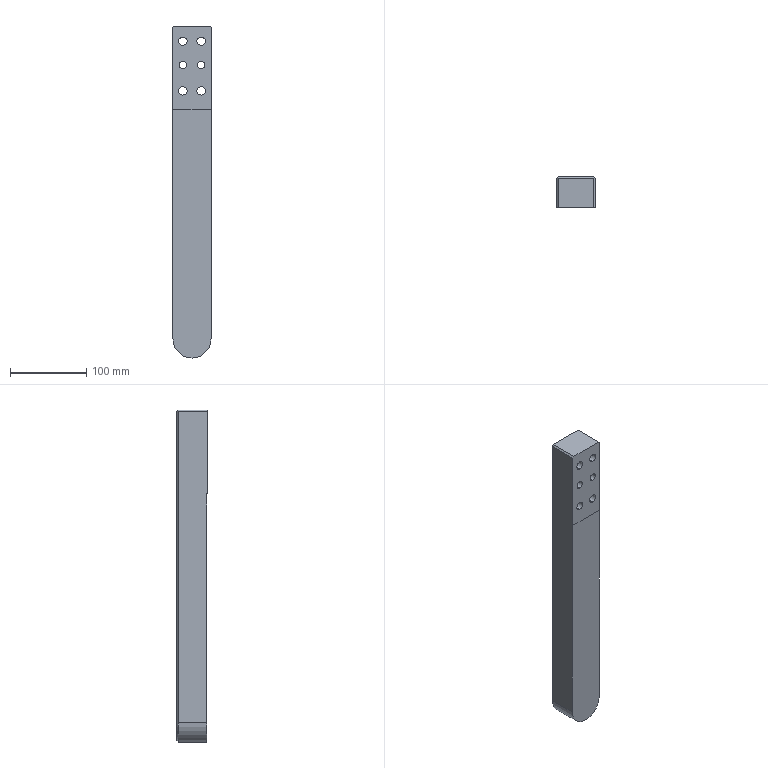Part | Creo | 1 solid | 38 faces | box 50 x 40 x 435 mm | volume 814187 mm3 | cylinder 21 | plane 16 | cone 1 | commonest cylinder face diameters 11 x8 16.8 x8 10 x4 50 x1
STEP:
#1=CARTESIAN_POINT('',(-135.,390.,-300.));
#2=VERTEX_POINT('',#1);
#3=CARTESIAN_POINT('',(-135.,390.,108.));
#4=VERTEX_POINT('',#3);
#5=CARTESIAN_POINT('',(-135.,390.,-300.));
#6=DIRECTION('',(0.,0.,1.));
#7=VECTOR('',#6,408.);
#8=LINE('',#5,#7);
#9=EDGE_CURVE('',#2,#4,#8,.T.);
#10=ORIENTED_EDGE('',*,*,#9,.T.);
#11=CARTESIAN_POINT('',(-181.,390.,108.));
#12=VERTEX_POINT('',#11);
#13=CARTESIAN_POINT('',(-135.,390.,108.));
#14=DIRECTION('',(-1.,0.,0.));
#15=VECTOR('',#14,46.);
#16=LINE('',#13,#15);
#17=EDGE_CURVE('',#4,#12,#16,.T.);
#18=ORIENTED_EDGE('',*,*,#17,.T.);
#19=CARTESIAN_POINT('',(-181.,390.,-300.));
#20=VERTEX_POINT('',#19);
#21=CARTESIAN_POINT('',(-181.,390.,108.));
#22=DIRECTION('',(0.,0.,-1.));
#23=VECTOR('',#22,408.);
#24=LINE('',#21,#23);
#25=EDGE_CURVE('',#12,#20,#24,.T.);
#26=ORIENTED_EDGE('',*,*,#25,.T.);
#27=CARTESIAN_POINT('',(-158.,390.,-323.));
#28=VERTEX_POINT('',#27);
#29=CARTESIAN_POINT('',(-158.,390.,-300.));
#30=DIRECTION('',(0.,1.,0.));
#31=DIRECTION('',(0.,0.,-1.));
#32=AXIS2_PLACEMENT_3D('',#29,#30,#31);
#33=CIRCLE('',#32,23.);
#34=EDGE_CURVE('',#28,#20,#33,.T.);
#35=ORIENTED_EDGE('',*,*,#34,.F.);
#36=CARTESIAN_POINT('',(-158.,390.,-300.));
#37=DIRECTION('',(0.,1.,0.));
#38=DIRECTION('',(1.,0.,-0.000000004));
#39=AXIS2_PLACEMENT_3D('',#36,#37,#38);
#40=CIRCLE('',#39,23.);
#41=EDGE_CURVE('',#2,#28,#40,.T.);
#42=ORIENTED_EDGE('',*,*,#41,.F.);
#43=EDGE_LOOP('',(#10,#18,#26,#35,#42));
#44=FACE_OUTER_BOUND('',#43,.F.);
#45=CARTESIAN_POINT('',(-154.4,390.,25.));
#46=VERTEX_POINT('',#45);
#47=CARTESIAN_POINT('',(-146.,390.,16.6));
#48=VERTEX_POINT('',#47);
#49=CARTESIAN_POINT('',(-146.,390.,25.));
#50=DIRECTION('',(0.,-1.,0.));
#51=DIRECTION('',(-1.,0.,0.));
#52=AXIS2_PLACEMENT_3D('',#49,#50,#51);
#53=CIRCLE('',#52,8.4);
#54=EDGE_CURVE('',#46,#48,#53,.T.);
#55=ORIENTED_EDGE('',*,*,#54,.F.);
#56=CARTESIAN_POINT('',(-146.,390.,33.4));
#57=VERTEX_POINT('',#56);
#58=CARTESIAN_POINT('',(-146.,390.,25.));
#59=DIRECTION('',(0.,-1.,0.));
#60=DIRECTION('',(0.,0.,1.));
#61=AXIS2_PLACEMENT_3D('',#58,#59,#60);
#62=CIRCLE('',#61,8.4);
#63=EDGE_CURVE('',#57,#46,#62,.T.);
#64=ORIENTED_EDGE('',*,*,#63,.F.);
#65=CARTESIAN_POINT('',(-146.,390.,25.));
#66=DIRECTION('',(0.,-1.,0.));
#67=DIRECTION('',(0.,0.,-1.));
#68=AXIS2_PLACEMENT_3D('',#65,#66,#67);
#69=CIRCLE('',#68,8.4);
#70=EDGE_CURVE('',#48,#57,#69,.T.);
#71=ORIENTED_EDGE('',*,*,#70,.F.);
#72=EDGE_LOOP('',(#55,#64,#71));
#73=FACE_BOUND('',#72,.F.);
#74=CARTESIAN_POINT('',(-178.4,390.,90.));
#75=VERTEX_POINT('',#74);
#76=CARTESIAN_POINT('',(-170.,390.,81.6));
#77=VERTEX_POINT('',#76);
#78=CARTESIAN_POINT('',(-170.,390.,90.));
#79=DIRECTION('',(0.,-1.,0.));
#80=DIRECTION('',(-1.,0.,0.));
#81=AXIS2_PLACEMENT_3D('',#78,#79,#80);
#82=CIRCLE('',#81,8.4);
#83=EDGE_CURVE('',#75,#77,#82,.T.);
#84=ORIENTED_EDGE('',*,*,#83,.F.);
#85=CARTESIAN_POINT('',(-170.,390.,98.4));
#86=VERTEX_POINT('',#85);
#87=CARTESIAN_POINT('',(-170.,390.,90.));
#88=DIRECTION('',(0.,-1.,0.));
#89=DIRECTION('',(0.,0.,1.));
#90=AXIS2_PLACEMENT_3D('',#87,#88,#89);
#91=CIRCLE('',#90,8.4);
#92=EDGE_CURVE('',#86,#75,#91,.T.);
#93=ORIENTED_EDGE('',*,*,#92,.F.);
#94=CARTESIAN_POINT('',(-170.,390.,90.));
#95=DIRECTION('',(0.,-1.,0.));
#96=DIRECTION('',(0.,0.,-1.));
#97=AXIS2_PLACEMENT_3D('',#94,#95,#96);
#98=CIRCLE('',#97,8.4);
#99=EDGE_CURVE('',#77,#86,#98,.T.);
#100=ORIENTED_EDGE('',*,*,#99,.F.);
#101=EDGE_LOOP('',(#84,#93,#100));
#102=FACE_BOUND('',#101,.F.);
#103=CARTESIAN_POINT('',(-178.4,390.,25.));
#104=VERTEX_POINT('',#103);
#105=CARTESIAN_POINT('',(-170.,390.,16.6));
#106=VERTEX_POINT('',#105);
#107=CARTESIAN_POINT('',(-170.,390.,25.));
#108=DIRECTION('',(0.,-1.,0.));
#109=DIRECTION('',(-1.,0.,0.));
#110=AXIS2_PLACEMENT_3D('',#107,#108,#109);
#111=CIRCLE('',#110,8.4);
#112=EDGE_CURVE('',#104,#106,#111,.T.);
#113=ORIENTED_EDGE('',*,*,#112,.F.);
#114=CARTESIAN_POINT('',(-170.,390.,33.4));
#115=VERTEX_POINT('',#114);
#116=CARTESIAN_POINT('',(-170.,390.,25.));
#117=DIRECTION('',(0.,-1.,0.));
#118=DIRECTION('',(0.,0.,1.));
#119=AXIS2_PLACEMENT_3D('',#116,#117,#118);
#120=CIRCLE('',#119,8.4);
#121=EDGE_CURVE('',#115,#104,#120,.T.);
#122=ORIENTED_EDGE('',*,*,#121,.F.);
#123=CARTESIAN_POINT('',(-170.,390.,25.));
#124=DIRECTION('',(0.,-1.,0.));
#125=DIRECTION('',(0.,0.,-1.));
#126=AXIS2_PLACEMENT_3D('',#123,#124,#125);
#127=CIRCLE('',#126,8.4);
#128=EDGE_CURVE('',#106,#115,#127,.T.);
#129=ORIENTED_EDGE('',*,*,#128,.F.);
#130=EDGE_LOOP('',(#113,#122,#129));
#131=FACE_BOUND('',#130,.F.);
#132=CARTESIAN_POINT('',(-154.4,390.,90.));
#133=VERTEX_POINT('',#132);
#134=CARTESIAN_POINT('',(-146.,390.,81.6));
#135=VERTEX_POINT('',#134);
#136=CARTESIAN_POINT('',(-146.,390.,90.));
#137=DIRECTION('',(0.,-1.,0.));
#138=DIRECTION('',(-1.,0.,0.));
#139=AXIS2_PLACEMENT_3D('',#136,#137,#138);
#140=CIRCLE('',#139,8.4);
#141=EDGE_CURVE('',#133,#135,#140,.T.);
#142=ORIENTED_EDGE('',*,*,#141,.F.);
#143=CARTESIAN_POINT('',(-146.,390.,98.4));
#144=VERTEX_POINT('',#143);
#145=CARTESIAN_POINT('',(-146.,390.,90.));
#146=DIRECTION('',(0.,-1.,0.));
#147=DIRECTION('',(0.,0.,1.));
#148=AXIS2_PLACEMENT_3D('',#145,#146,#147);
#149=CIRCLE('',#148,8.4);
#150=EDGE_CURVE('',#144,#133,#149,.T.);
#151=ORIENTED_EDGE('',*,*,#150,.F.);
#152=CARTESIAN_POINT('',(-146.,390.,90.));
#153=DIRECTION('',(0.,-1.,0.));
#154=DIRECTION('',(0.,0.,-1.));
#155=AXIS2_PLACEMENT_3D('',#152,#153,#154);
#156=CIRCLE('',#155,8.4);
#157=EDGE_CURVE('',#135,#144,#156,.T.);
#158=ORIENTED_EDGE('',*,*,#157,.F.);
#159=EDGE_LOOP('',(#142,#151,#158));
#160=FACE_BOUND('',#159,.F.);
#161=CARTESIAN_POINT('',(-170.,390.,54.));
#162=VERTEX_POINT('',#161);
#163=CARTESIAN_POINT('',(-170.,390.,64.));
#164=VERTEX_POINT('',#163);
#165=CARTESIAN_POINT('',(-170.,390.,59.));
#166=DIRECTION('',(0.,-1.,0.));
#167=DIRECTION('',(0.,0.,-1.));
#168=AXIS2_PLACEMENT_3D('',#165,#166,#167);
#169=CIRCLE('',#168,5.);
#170=EDGE_CURVE('',#162,#164,#169,.T.);
#171=ORIENTED_EDGE('',*,*,#170,.F.);
#172=CARTESIAN_POINT('',(-170.,390.,59.));
#173=DIRECTION('',(0.,-1.,0.));
#174=DIRECTION('',(0.,0.,1.));
#175=AXIS2_PLACEMENT_3D('',#172,#173,#174);
#176=CIRCLE('',#175,5.);
#177=EDGE_CURVE('',#164,#162,#176,.T.);
#178=ORIENTED_EDGE('',*,*,#177,.F.);
#179=EDGE_LOOP('',(#171,#178));
#180=FACE_BOUND('',#179,.F.);
#181=CARTESIAN_POINT('',(-146.,390.,54.));
#182=VERTEX_POINT('',#181);
#183=CARTESIAN_POINT('',(-146.,390.,64.));
#184=VERTEX_POINT('',#183);
#185=CARTESIAN_POINT('',(-146.,390.,59.));
#186=DIRECTION('',(0.,-1.,0.));
#187=DIRECTION('',(0.,0.,-1.));
#188=AXIS2_PLACEMENT_3D('',#185,#186,#187);
#189=CIRCLE('',#188,5.);
#190=EDGE_CURVE('',#182,#184,#189,.T.);
#191=ORIENTED_EDGE('',*,*,#190,.F.);
#192=CARTESIAN_POINT('',(-146.,390.,59.));
#193=DIRECTION('',(0.,-1.,0.));
#194=DIRECTION('',(0.,0.,1.));
#195=AXIS2_PLACEMENT_3D('',#192,#193,#194);
#196=CIRCLE('',#195,5.);
#197=EDGE_CURVE('',#184,#182,#196,.T.);
#198=ORIENTED_EDGE('',*,*,#197,.F.);
#199=EDGE_LOOP('',(#191,#198));
#200=FACE_BOUND('',#199,.F.);
#201=CARTESIAN_POINT('',(322.,390.,50.));
#202=DIRECTION('',(0.,1.,0.));
#203=DIRECTION('',(0.,0.,-1.));
#204=AXIS2_PLACEMENT_3D('',#201,#202,#203);
#205=PLANE('',#204);
#206=ADVANCED_FACE('',(#44,#73,#102,#131,#160,#180,#200),#205,.T.);
#207=ORIENTED_EDGE('',*,*,#150,.T.);
#208=ORIENTED_EDGE('',*,*,#141,.T.);
#209=CARTESIAN_POINT('',(-146.,379.,81.6));
#210=VERTEX_POINT('',#209);
#211=CARTESIAN_POINT('',(-146.,379.,81.6));
#212=DIRECTION('',(0.,1.,0.));
#213=VECTOR('',#212,11.);
#214=LINE('',#211,#213);
#215=EDGE_CURVE('',#210,#135,#214,.T.);
#216=ORIENTED_EDGE('',*,*,#215,.F.);
#217=CARTESIAN_POINT('',(-154.4,379.,90.));
#218=VERTEX_POINT('',#217);
#219=CARTESIAN_POINT('',(-146.,379.,90.));
#220=DIRECTION('',(0.,1.,0.));
#221=DIRECTION('',(0.,0.,-1.));
#222=AXIS2_PLACEMENT_3D('',#219,#220,#221);
#223=CIRCLE('',#222,8.4);
#224=EDGE_CURVE('',#210,#218,#223,.T.);
#225=ORIENTED_EDGE('',*,*,#224,.T.);
#226=CARTESIAN_POINT('',(-146.,379.,98.4));
#227=VERTEX_POINT('',#226);
#228=CARTESIAN_POINT('',(-146.,379.,90.));
#229=DIRECTION('',(0.,1.,0.));
#230=DIRECTION('',(-1.,0.,0.));
#231=AXIS2_PLACEMENT_3D('',#228,#229,#230);
#232=CIRCLE('',#231,8.4);
#233=EDGE_CURVE('',#218,#227,#232,.T.);
#234=ORIENTED_EDGE('',*,*,#233,.T.);
#235=CARTESIAN_POINT('',(-146.,379.,98.4));
#236=DIRECTION('',(0.,1.,0.));
#237=VECTOR('',#236,11.);
#238=LINE('',#235,#237);
#239=EDGE_CURVE('',#227,#144,#238,.T.);
#240=ORIENTED_EDGE('',*,*,#239,.T.);
#241=EDGE_LOOP('',(#207,#208,#216,#225,#234,#240));
#242=FACE_OUTER_BOUND('',#241,.F.);
#243=CARTESIAN_POINT('',(-146.,379.,90.));
#244=DIRECTION('',(0.,1.,0.));
#245=DIRECTION('',(0.,0.,-1.));
#246=AXIS2_PLACEMENT_3D('',#243,#244,#245);
#247=CYLINDRICAL_SURFACE('',#246,8.4);
#248=ADVANCED_FACE('',(#242),#247,.F.);
#249=ORIENTED_EDGE('',*,*,#157,.T.);
#250=ORIENTED_EDGE('',*,*,#239,.F.);
#251=CARTESIAN_POINT('',(-137.6,379.,90.));
#252=VERTEX_POINT('',#251);
#253=CARTESIAN_POINT('',(-146.,379.,90.));
#254=DIRECTION('',(0.,1.,0.));
#255=DIRECTION('',(0.,0.,1.));
#256=AXIS2_PLACEMENT_3D('',#253,#254,#255);
#257=CIRCLE('',#256,8.4);
#258=EDGE_CURVE('',#227,#252,#257,.T.);
#259=ORIENTED_EDGE('',*,*,#258,.T.);
#260=CARTESIAN_POINT('',(-146.,379.,90.));
#261=DIRECTION('',(0.,1.,0.));
#262=DIRECTION('',(1.,0.,0.));
#263=AXIS2_PLACEMENT_3D('',#260,#261,#262);
#264=CIRCLE('',#263,8.4);
#265=EDGE_CURVE('',#252,#210,#264,.T.);
#266=ORIENTED_EDGE('',*,*,#265,.T.);
#267=ORIENTED_EDGE('',*,*,#215,.T.);
#268=EDGE_LOOP('',(#249,#250,#259,#266,#267));
#269=FACE_OUTER_BOUND('',#268,.F.);
#270=CARTESIAN_POINT('',(-146.,379.,90.));
#271=DIRECTION('',(0.,1.,0.));
#272=DIRECTION('',(0.,0.,-1.));
#273=AXIS2_PLACEMENT_3D('',#270,#271,#272);
#274=CYLINDRICAL_SURFACE('',#273,8.4);
#275=ADVANCED_FACE('',(#269),#274,.F.);
#276=ORIENTED_EDGE('',*,*,#233,.F.);
#277=ORIENTED_EDGE('',*,*,#224,.F.);
#278=ORIENTED_EDGE('',*,*,#265,.F.);
#279=ORIENTED_EDGE('',*,*,#258,.F.);
#280=EDGE_LOOP('',(#276,#277,#278,#279));
#281=FACE_OUTER_BOUND('',#280,.F.);
#282=CARTESIAN_POINT('',(-146.,379.,84.5));
#283=VERTEX_POINT('',#282);
#284=CARTESIAN_POINT('',(-146.,379.,95.5));
#285=VERTEX_POINT('',#284);
#286=CARTESIAN_POINT('',(-146.,379.,90.));
#287=DIRECTION('',(0.,-1.,0.));
#288=DIRECTION('',(0.,0.,-1.));
#289=AXIS2_PLACEMENT_3D('',#286,#287,#288);
#290=CIRCLE('',#289,5.5);
#291=EDGE_CURVE('',#283,#285,#290,.T.);
#292=ORIENTED_EDGE('',*,*,#291,.F.);
#293=CARTESIAN_POINT('',(-146.,379.,90.));
#294=DIRECTION('',(0.,-1.,0.));
#295=DIRECTION('',(0.,0.,1.));
#296=AXIS2_PLACEMENT_3D('',#293,#294,#295);
#297=CIRCLE('',#296,5.5);
#298=EDGE_CURVE('',#285,#283,#297,.T.);
#299=ORIENTED_EDGE('',*,*,#298,.F.);
#300=EDGE_LOOP('',(#292,#299));
#301=FACE_BOUND('',#300,.F.);
#302=CARTESIAN_POINT('',(22.,379.,-0.5));
#303=DIRECTION('',(0.,1.,0.));
#304=DIRECTION('',(0.,0.,-1.));
#305=AXIS2_PLACEMENT_3D('',#302,#303,#304);
#306=PLANE('',#305);
#307=ADVANCED_FACE('',(#281,#301),#306,.T.);
#308=CARTESIAN_POINT('',(-146.,350.,95.5));
#309=VERTEX_POINT('',#308);
#310=CARTESIAN_POINT('',(-146.,350.,84.5));
#311=VERTEX_POINT('',#310);
#312=CARTESIAN_POINT('',(-146.,350.,90.));
#313=DIRECTION('',(0.,1.,0.));
#314=DIRECTION('',(0.,0.,1.));
#315=AXIS2_PLACEMENT_3D('',#312,#313,#314);
#316=CIRCLE('',#315,5.5);
#317=EDGE_CURVE('',#309,#311,#316,.T.);
#318=ORIENTED_EDGE('',*,*,#317,.T.);
#319=CARTESIAN_POINT('',(-146.,350.,84.5));
#320=DIRECTION('',(0.,1.,0.));
#321=VECTOR('',#320,29.);
#322=LINE('',#319,#321);
#323=EDGE_CURVE('',#311,#283,#322,.T.);
#324=ORIENTED_EDGE('',*,*,#323,.T.);
#325=ORIENTED_EDGE('',*,*,#291,.T.);
#326=CARTESIAN_POINT('',(-146.,350.,95.5));
#327=DIRECTION('',(0.,1.,0.));
#328=VECTOR('',#327,29.);
#329=LINE('',#326,#328);
#330=EDGE_CURVE('',#309,#285,#329,.T.);
#331=ORIENTED_EDGE('',*,*,#330,.F.);
#332=EDGE_LOOP('',(#318,#324,#325,#331));
#333=FACE_OUTER_BOUND('',#332,.F.);
#334=CARTESIAN_POINT('',(-146.,390.,90.));
#335=DIRECTION('',(0.,1.,0.));
#336=DIRECTION('',(0.,0.,-1.));
#337=AXIS2_PLACEMENT_3D('',#334,#335,#336);
#338=CYLINDRICAL_SURFACE('',#337,5.5);
#339=ADVANCED_FACE('',(#333),#338,.F.);
#340=CARTESIAN_POINT('',(-133.,350.,0.));
#341=VERTEX_POINT('',#340);
#342=CARTESIAN_POINT('',(-133.,350.,108.));
#343=VERTEX_POINT('',#342);
#344=CARTESIAN_POINT('',(-133.,350.,0.));
#345=DIRECTION('',(0.,0.,1.));
#346=VECTOR('',#345,108.);
#347=LINE('',#344,#346);
#348=EDGE_CURVE('',#341,#343,#347,.T.);
#349=ORIENTED_EDGE('',*,*,#348,.F.);
#350=CARTESIAN_POINT('',(-183.,350.,0.));
#351=VERTEX_POINT('',#350);
#352=CARTESIAN_POINT('',(-183.,350.,0.));
#353=DIRECTION('',(1.,0.,0.));
#354=VECTOR('',#353,50.);
#355=LINE('',#352,#354);
#356=EDGE_CURVE('',#351,#341,#355,.T.);
#357=ORIENTED_EDGE('',*,*,#356,.F.);
#358=CARTESIAN_POINT('',(-183.,350.,108.));
#359=VERTEX_POINT('',#358);
#360=CARTESIAN_POINT('',(-183.,350.,108.));
#361=DIRECTION('',(0.,0.,-1.));
#362=VECTOR('',#361,108.);
#363=LINE('',#360,#362);
#364=EDGE_CURVE('',#359,#351,#363,.T.);
#365=ORIENTED_EDGE('',*,*,#364,.F.);
#366=CARTESIAN_POINT('',(-181.,350.,110.));
#367=VERTEX_POINT('',#366);
#368=CARTESIAN_POINT('',(-181.,350.,110.));
#369=DIRECTION('',(-0.7071,0.,-0.7071));
#370=VECTOR('',#369,2.828);
#371=LINE('',#368,#370);
#372=EDGE_CURVE('',#367,#359,#371,.T.);
#373=ORIENTED_EDGE('',*,*,#372,.F.);
#374=CARTESIAN_POINT('',(-135.,350.,110.));
#375=VERTEX_POINT('',#374);
#376=CARTESIAN_POINT('',(-135.,350.,110.));
#377=DIRECTION('',(-1.,0.,0.));
#378=VECTOR('',#377,46.);
#379=LINE('',#376,#378);
#380=EDGE_CURVE('',#375,#367,#379,.T.);
#381=ORIENTED_EDGE('',*,*,#380,.F.);
#382=CARTESIAN_POINT('',(-133.,350.,108.));
#383=DIRECTION('',(-0.7071,0.,0.7071));
#384=VECTOR('',#383,2.828);
#385=LINE('',#382,#384);
#386=EDGE_CURVE('',#343,#375,#385,.T.);
#387=ORIENTED_EDGE('',*,*,#386,.F.);
#388=EDGE_LOOP('',(#349,#357,#365,#373,#381,#387));
#389=FACE_OUTER_BOUND('',#388,.F.);
#390=CARTESIAN_POINT('',(-146.,350.,90.));
#391=DIRECTION('',(0.,1.,0.));
#392=DIRECTION('',(0.,0.,-1.));
#393=AXIS2_PLACEMENT_3D('',#390,#391,#392);
#394=CIRCLE('',#393,5.5);
#395=EDGE_CURVE('',#311,#309,#394,.T.);
#396=ORIENTED_EDGE('',*,*,#395,.F.);
#397=ORIENTED_EDGE('',*,*,#317,.F.);
#398=EDGE_LOOP('',(#396,#397));
#399=FACE_BOUND('',#398,.F.);
#400=CARTESIAN_POINT('',(-170.,350.,19.5));
#401=VERTEX_POINT('',#400);
#402=CARTESIAN_POINT('',(-170.,350.,30.5));
#403=VERTEX_POINT('',#402);
#404=CARTESIAN_POINT('',(-170.,350.,25.));
#405=DIRECTION('',(0.,1.,0.));
#406=DIRECTION('',(0.,0.,-1.));
#407=AXIS2_PLACEMENT_3D('',#404,#405,#406);
#408=CIRCLE('',#407,5.5);
#409=EDGE_CURVE('',#401,#403,#408,.T.);
#410=ORIENTED_EDGE('',*,*,#409,.F.);
#411=CARTESIAN_POINT('',(-170.,350.,25.));
#412=DIRECTION('',(0.,1.,0.));
#413=DIRECTION('',(0.,0.,1.));
#414=AXIS2_PLACEMENT_3D('',#411,#412,#413);
#415=CIRCLE('',#414,5.5);
#416=EDGE_CURVE('',#403,#401,#415,.T.);
#417=ORIENTED_EDGE('',*,*,#416,.F.);
#418=EDGE_LOOP('',(#410,#417));
#419=FACE_BOUND('',#418,.F.);
#420=CARTESIAN_POINT('',(-146.,350.,19.5));
#421=VERTEX_POINT('',#420);
#422=CARTESIAN_POINT('',(-146.,350.,30.5));
#423=VERTEX_POINT('',#422);
#424=CARTESIAN_POINT('',(-146.,350.,25.));
#425=DIRECTION('',(0.,1.,0.));
#426=DIRECTION('',(0.,0.,-1.));
#427=AXIS2_PLACEMENT_3D('',#424,#425,#426);
#428=CIRCLE('',#427,5.5);
#429=EDGE_CURVE('',#421,#423,#428,.T.);
#430=ORIENTED_EDGE('',*,*,#429,.F.);
#431=CARTESIAN_POINT('',(-146.,350.,25.));
#432=DIRECTION('',(0.,1.,0.));
#433=DIRECTION('',(0.,0.,1.));
#434=AXIS2_PLACEMENT_3D('',#431,#432,#433);
#435=CIRCLE('',#434,5.5);
#436=EDGE_CURVE('',#423,#421,#435,.T.);
#437=ORIENTED_EDGE('',*,*,#436,.F.);
#438=EDGE_LOOP('',(#430,#437));
#439=FACE_BOUND('',#438,.F.);
#440=CARTESIAN_POINT('',(-170.,350.,84.5));
#441=VERTEX_POINT('',#440);
#442=CARTESIAN_POINT('',(-170.,350.,95.5));
#443=VERTEX_POINT('',#442);
#444=CARTESIAN_POINT('',(-170.,350.,90.));
#445=DIRECTION('',(0.,1.,0.));
#446=DIRECTION('',(0.,0.,-1.));
#447=AXIS2_PLACEMENT_3D('',#444,#445,#446);
#448=CIRCLE('',#447,5.5);
#449=EDGE_CURVE('',#441,#443,#448,.T.);
#450=ORIENTED_EDGE('',*,*,#449,.F.);
#451=CARTESIAN_POINT('',(-170.,350.,90.));
#452=DIRECTION('',(0.,1.,0.));
#453=DIRECTION('',(0.,0.,1.));
#454=AXIS2_PLACEMENT_3D('',#451,#452,#453);
#455=CIRCLE('',#454,5.5);
#456=EDGE_CURVE('',#443,#441,#455,.T.);
#457=ORIENTED_EDGE('',*,*,#456,.F.);
#458=EDGE_LOOP('',(#450,#457));
#459=FACE_BOUND('',#458,.F.);
#460=CARTESIAN_POINT('',(-170.,350.,54.));
#461=VERTEX_POINT('',#460);
#462=CARTESIAN_POINT('',(-170.,350.,64.));
#463=VERTEX_POINT('',#462);
#464=CARTESIAN_POINT('',(-170.,350.,59.));
#465=DIRECTION('',(0.,1.,0.));
#466=DIRECTION('',(0.,0.,-1.));
#467=AXIS2_PLACEMENT_3D('',#464,#465,#466);
#468=CIRCLE('',#467,5.);
#469=EDGE_CURVE('',#461,#463,#468,.T.);
#470=ORIENTED_EDGE('',*,*,#469,.F.);
#471=CARTESIAN_POINT('',(-170.,350.,59.));
#472=DIRECTION('',(0.,1.,0.));
#473=DIRECTION('',(0.,0.,1.));
#474=AXIS2_PLACEMENT_3D('',#471,#472,#473);
#475=CIRCLE('',#474,5.);
#476=EDGE_CURVE('',#463,#461,#475,.T.);
#477=ORIENTED_EDGE('',*,*,#476,.F.);
#478=EDGE_LOOP('',(#470,#477));
#479=FACE_BOUND('',#478,.F.);
#480=CARTESIAN_POINT('',(-146.,350.,54.));
#481=VERTEX_POINT('',#480);
#482=CARTESIAN_POINT('',(-146.,350.,64.));
#483=VERTEX_POINT('',#482);
#484=CARTESIAN_POINT('',(-146.,350.,59.));
#485=DIRECTION('',(0.,1.,0.));
#486=DIRECTION('',(0.,0.,-1.));
#487=AXIS2_PLACEMENT_3D('',#484,#485,#486);
#488=CIRCLE('',#487,5.);
#489=EDGE_CURVE('',#481,#483,#488,.T.);
#490=ORIENTED_EDGE('',*,*,#489,.F.);
#491=CARTESIAN_POINT('',(-146.,350.,59.));
#492=DIRECTION('',(0.,1.,0.));
#493=DIRECTION('',(0.,0.,1.));
#494=AXIS2_PLACEMENT_3D('',#491,#492,#493);
#495=CIRCLE('',#494,5.);
#496=EDGE_CURVE('',#483,#481,#495,.T.);
#497=ORIENTED_EDGE('',*,*,#496,.F.);
#498=EDGE_LOOP('',(#490,#497));
#499=FACE_BOUND('',#498,.F.);
#500=CARTESIAN_POINT('',(322.,350.,0.));
#501=DIRECTION('',(0.,1.,0.));
#502=DIRECTION('',(0.,0.,-1.));
#503=AXIS2_PLACEMENT_3D('',#500,#501,#502);
#504=PLANE('',#503);
#505=ADVANCED_FACE('',(#389,#399,#419,#439,#459,#479,#499),#504,.F.);
#506=CARTESIAN_POINT('',(-133.,351.,0.));
#507=VERTEX_POINT('',#506);
#508=CARTESIAN_POINT('',(-133.,351.,-300.));
#509=VERTEX_POINT('',#508);
#510=CARTESIAN_POINT('',(-133.,351.,0.));
#511=DIRECTION('',(0.,0.,-1.));
#512=VECTOR('',#511,300.);
#513=LINE('',#510,#512);
#514=EDGE_CURVE('',#507,#509,#513,.T.);
#515=ORIENTED_EDGE('',*,*,#514,.F.);
#516=CARTESIAN_POINT('',(-133.,351.,0.));
#517=DIRECTION('',(0.,-1.,0.));
#518=VECTOR('',#517,1.);
#519=LINE('',#516,#518);
#520=EDGE_CURVE('',#507,#341,#519,.T.);
#521=ORIENTED_EDGE('',*,*,#520,.T.);
#522=ORIENTED_EDGE('',*,*,#348,.T.);
#523=CARTESIAN_POINT('',(-133.,388.,108.));
#524=VERTEX_POINT('',#523);
#525=CARTESIAN_POINT('',(-133.,350.,108.));
#526=DIRECTION('',(0.,1.,0.));
#527=VECTOR('',#526,38.);
#528=LINE('',#525,#527);
#529=EDGE_CURVE('',#343,#524,#528,.T.);
#530=ORIENTED_EDGE('',*,*,#529,.T.);
#531=CARTESIAN_POINT('',(-133.,388.,-300.));
#532=VERTEX_POINT('',#531);
#533=CARTESIAN_POINT('',(-133.,388.,-300.));
#534=DIRECTION('',(0.,0.,1.));
#535=VECTOR('',#534,408.);
#536=LINE('',#533,#535);
#537=EDGE_CURVE('',#532,#524,#536,.T.);
#538=ORIENTED_EDGE('',*,*,#537,.F.);
#539=CARTESIAN_POINT('',(-133.,388.,-300.));
#540=DIRECTION('',(0.,-1.,0.));
#541=VECTOR('',#540,37.);
#542=LINE('',#539,#541);
#543=EDGE_CURVE('',#532,#509,#542,.T.);
#544=ORIENTED_EDGE('',*,*,#543,.T.);
#545=EDGE_LOOP('',(#515,#521,#522,#530,#538,#544));
#546=FACE_OUTER_BOUND('',#545,.F.);
#547=CARTESIAN_POINT('',(-133.,350.,160.));
#548=DIRECTION('',(1.,0.,0.));
#549=DIRECTION('',(0.,0.,1.));
#550=AXIS2_PLACEMENT_3D('',#547,#548,#549);
#551=PLANE('',#550);
#552=ADVANCED_FACE('',(#546),#551,.T.);
#553=ORIENTED_EDGE('',*,*,#514,.T.);
#554=CARTESIAN_POINT('',(-158.,351.,-325.));
#555=VERTEX_POINT('',#554);
#556=CARTESIAN_POINT('',(-158.,351.,-300.));
#557=DIRECTION('',(0.,-1.,0.));
#558=DIRECTION('',(0.,0.,-1.));
#559=AXIS2_PLACEMENT_3D('',#556,#557,#558);
#560=CIRCLE('',#559,25.);
#561=EDGE_CURVE('',#555,#509,#560,.T.);
#562=ORIENTED_EDGE('',*,*,#561,.F.);
#563=CARTESIAN_POINT('',(-183.,351.,-300.));
#564=VERTEX_POINT('',#563);
#565=CARTESIAN_POINT('',(-158.,351.,-300.));
#566=DIRECTION('',(0.,-1.,0.));
#567=DIRECTION('',(-1.,0.,0.));
#568=AXIS2_PLACEMENT_3D('',#565,#566,#567);
#569=CIRCLE('',#568,25.);
#570=EDGE_CURVE('',#564,#555,#569,.T.);
#571=ORIENTED_EDGE('',*,*,#570,.F.);
#572=CARTESIAN_POINT('',(-183.,351.,0.));
#573=VERTEX_POINT('',#572);
#574=CARTESIAN_POINT('',(-183.,351.,0.));
#575=DIRECTION('',(0.,0.,-1.));
#576=VECTOR('',#575,300.);
#577=LINE('',#574,#576);
#578=EDGE_CURVE('',#573,#564,#577,.T.);
#579=ORIENTED_EDGE('',*,*,#578,.F.);
#580=CARTESIAN_POINT('',(-133.,351.,0.));
#581=DIRECTION('',(-1.,0.,0.));
#582=VECTOR('',#581,50.);
#583=LINE('',#580,#582);
#584=EDGE_CURVE('',#507,#573,#583,.T.);
#585=ORIENTED_EDGE('',*,*,#584,.F.);
#586=EDGE_LOOP('',(#553,#562,#571,#579,#585));
#587=FACE_OUTER_BOUND('',#586,.F.);
#588=CARTESIAN_POINT('',(-183.,351.,50.));
#589=DIRECTION('',(0.,1.,0.));
#590=DIRECTION('',(0.,0.,-1.));
#591=AXIS2_PLACEMENT_3D('',#588,#589,#590);
#592=PLANE('',#591);
#593=ADVANCED_FACE('',(#587),#592,.F.);
#594=CARTESIAN_POINT('',(-183.,388.,-300.));
#595=VERTEX_POINT('',#594);
#596=CARTESIAN_POINT('',(-183.,351.,-300.));
#597=DIRECTION('',(0.,1.,0.));
#598=VECTOR('',#597,37.);
#599=LINE('',#596,#598);
#600=EDGE_CURVE('',#564,#595,#599,.T.);
#601=ORIENTED_EDGE('',*,*,#600,.F.);
#602=ORIENTED_EDGE('',*,*,#570,.T.);
#603=ORIENTED_EDGE('',*,*,#561,.T.);
#604=ORIENTED_EDGE('',*,*,#543,.F.);
#605=CARTESIAN_POINT('',(-158.,388.,-325.));
#606=VERTEX_POINT('',#605);
#607=CARTESIAN_POINT('',(-158.,388.,-300.));
#608=DIRECTION('',(0.,1.,0.));
#609=DIRECTION('',(1.,0.,0.));
#610=AXIS2_PLACEMENT_3D('',#607,#608,#609);
#611=CIRCLE('',#610,25.);
#612=EDGE_CURVE('',#532,#606,#611,.T.);
#613=ORIENTED_EDGE('',*,*,#612,.T.);
#614=CARTESIAN_POINT('',(-158.,388.,-300.));
#615=DIRECTION('',(0.,1.,0.));
#616=DIRECTION('',(0.,0.,-1.));
#617=AXIS2_PLACEMENT_3D('',#614,#615,#616);
#618=CIRCLE('',#617,25.);
#619=EDGE_CURVE('',#606,#595,#618,.T.);
#620=ORIENTED_EDGE('',*,*,#619,.T.);
#621=EDGE_LOOP('',(#601,#602,#603,#604,#613,#620));
#622=FACE_OUTER_BOUND('',#621,.F.);
#623=CARTESIAN_POINT('',(-158.,350.,-300.));
#624=DIRECTION('',(0.,1.,0.));
#625=DIRECTION('',(0.,0.,-1.));
#626=AXIS2_PLACEMENT_3D('',#623,#624,#625);
#627=CYLINDRICAL_SURFACE('',#626,25.);
#628=ADVANCED_FACE('',(#622),#627,.T.);
#629=ORIENTED_EDGE('',*,*,#364,.T.);
#630=CARTESIAN_POINT('',(-183.,351.,0.));
#631=DIRECTION('',(0.,-1.,0.));
#632=VECTOR('',#631,1.);
#633=LINE('',#630,#632);
#634=EDGE_CURVE('',#573,#351,#633,.T.);
#635=ORIENTED_EDGE('',*,*,#634,.F.);
#636=ORIENTED_EDGE('',*,*,#578,.T.);
#637=ORIENTED_EDGE('',*,*,#600,.T.);
#638=CARTESIAN_POINT('',(-183.,388.,108.));
#639=VERTEX_POINT('',#638);
#640=CARTESIAN_POINT('',(-183.,388.,108.));
#641=DIRECTION('',(0.,0.,-1.));
#642=VECTOR('',#641,408.);
#643=LINE('',#640,#642);
#644=EDGE_CURVE('',#639,#595,#643,.T.);
#645=ORIENTED_EDGE('',*,*,#644,.F.);
#646=CARTESIAN_POINT('',(-183.,350.,108.));
#647=DIRECTION('',(0.,1.,0.));
#648=VECTOR('',#647,38.);
#649=LINE('',#646,#648);
#650=EDGE_CURVE('',#359,#639,#649,.T.);
#651=ORIENTED_EDGE('',*,*,#650,.F.);
#652=EDGE_LOOP('',(#629,#635,#636,#637,#645,#651));
#653=FACE_OUTER_BOUND('',#652,.F.);
#654=CARTESIAN_POINT('',(-183.,350.,-285.));
#655=DIRECTION('',(-1.,0.,0.));
#656=DIRECTION('',(0.,0.,-1.));
#657=AXIS2_PLACEMENT_3D('',#654,#655,#656);
#658=PLANE('',#657);
#659=ADVANCED_FACE('',(#653),#658,.T.);
#660=ORIENTED_EDGE('',*,*,#634,.T.);
#661=ORIENTED_EDGE('',*,*,#356,.T.);
#662=ORIENTED_EDGE('',*,*,#520,.F.);
#663=ORIENTED_EDGE('',*,*,#584,.T.);
#664=EDGE_LOOP('',(#660,#661,#662,#663));
#665=FACE_OUTER_BOUND('',#664,.F.);
#666=CARTESIAN_POINT('',(-183.,350.,0.));
#667=DIRECTION('',(0.,0.,1.));
#668=DIRECTION('',(-1.,0.,0.));
#669=AXIS2_PLACEMENT_3D('',#666,#667,#668);
#670=PLANE('',#669);
#671=ADVANCED_FACE('',(#665),#670,.F.);
#672=CARTESIAN_POINT('',(-182.,389.,109.));
#673=VERTEX_POINT('',#672);
#674=CARTESIAN_POINT('',(-183.,388.,108.));
#675=DIRECTION('',(0.5774,0.5774,0.5774));
#676=VECTOR('',#675,1.732);
#677=LINE('',#674,#676);
#678=EDGE_CURVE('',#639,#673,#677,.T.);
#679=ORIENTED_EDGE('',*,*,#678,.F.);
#680=ORIENTED_EDGE('',*,*,#644,.T.);
#681=CARTESIAN_POINT('',(-183.,388.,-300.));
#682=DIRECTION('',(0.7071,0.7071,-0.000000016));
#683=VECTOR('',#682,2.828);
#684=LINE('',#681,#683);
#685=EDGE_CURVE('',#595,#20,#684,.T.);
#686=ORIENTED_EDGE('',*,*,#685,.T.);
#687=ORIENTED_EDGE('',*,*,#25,.F.);
#688=CARTESIAN_POINT('',(-182.,389.,109.));
#689=DIRECTION('',(0.5774,0.5774,-0.5774));
#690=VECTOR('',#689,1.732);
#691=LINE('',#688,#690);
#692=EDGE_CURVE('',#673,#12,#691,.T.);
#693=ORIENTED_EDGE('',*,*,#692,.F.);
#694=EDGE_LOOP('',(#679,#680,#686,#687,#693));
#695=FACE_OUTER_BOUND('',#694,.F.);
#696=CARTESIAN_POINT('',(-182.,389.,-62.5));
#697=DIRECTION('',(-0.7071,0.7071,0.));
#698=DIRECTION('',(-0.7071,-0.7071,0.));
#699=AXIS2_PLACEMENT_3D('',#696,#697,#698);
#700=PLANE('',#699);
#701=ADVANCED_FACE('',(#695),#700,.T.);
#702=CARTESIAN_POINT('',(-181.,388.,110.));
#703=VERTEX_POINT('',#702);
#704=CARTESIAN_POINT('',(-181.,350.,110.));
#705=DIRECTION('',(0.,1.,0.));
#706=VECTOR('',#705,38.);
#707=LINE('',#704,#706);
#708=EDGE_CURVE('',#367,#703,#707,.T.);
#709=ORIENTED_EDGE('',*,*,#708,.F.);
#710=ORIENTED_EDGE('',*,*,#372,.T.);
#711=ORIENTED_EDGE('',*,*,#650,.T.);
#712=ORIENTED_EDGE('',*,*,#678,.T.);
#713=CARTESIAN_POINT('',(-182.,389.,109.));
#714=DIRECTION('',(0.5774,-0.5774,0.5774));
#715=VECTOR('',#714,1.732);
#716=LINE('',#713,#715);
#717=EDGE_CURVE('',#673,#703,#716,.T.);
#718=ORIENTED_EDGE('',*,*,#717,.T.);
#719=EDGE_LOOP('',(#709,#710,#711,#712,#718));
#720=FACE_OUTER_BOUND('',#719,.F.);
#721=CARTESIAN_POINT('',(-182.,370.,109.));
#722=DIRECTION('',(-0.7071,0.,0.7071));
#723=DIRECTION('',(-0.7071,0.,-0.7071));
#724=AXIS2_PLACEMENT_3D('',#721,#722,#723);
#725=PLANE('',#724);
#726=ADVANCED_FACE('',(#720),#725,.T.);
#727=ORIENTED_EDGE('',*,*,#708,.T.);
#728=CARTESIAN_POINT('',(-135.,388.,110.));
#729=VERTEX_POINT('',#728);
#730=CARTESIAN_POINT('',(-135.,388.,110.));
#731=DIRECTION('',(-1.,0.,0.));
#732=VECTOR('',#731,46.);
#733=LINE('',#730,#732);
#734=EDGE_CURVE('',#729,#703,#733,.T.);
#735=ORIENTED_EDGE('',*,*,#734,.F.);
#736=CARTESIAN_POINT('',(-135.,350.,110.));
#737=DIRECTION('',(0.,1.,0.));
#738=VECTOR('',#737,38.);
#739=LINE('',#736,#738);
#740=EDGE_CURVE('',#375,#729,#739,.T.);
#741=ORIENTED_EDGE('',*,*,#740,.F.);
#742=ORIENTED_EDGE('',*,*,#380,.T.);
#743=EDGE_LOOP('',(#727,#735,#741,#742));
#744=FACE_OUTER_BOUND('',#743,.F.);
#745=CARTESIAN_POINT('',(-183.,350.,110.));
#746=DIRECTION('',(0.,0.,1.));
#747=DIRECTION('',(-1.,0.,0.));
#748=AXIS2_PLACEMENT_3D('',#745,#746,#747);
#749=PLANE('',#748);
#750=ADVANCED_FACE('',(#744),#749,.T.);
#751=CARTESIAN_POINT('',(-134.,389.,109.));
#752=VERTEX_POINT('',#751);
#753=CARTESIAN_POINT('',(-135.,388.,110.));
#754=DIRECTION('',(0.5774,0.5774,-0.5774));
#755=VECTOR('',#754,1.732);
#756=LINE('',#753,#755);
#757=EDGE_CURVE('',#729,#752,#756,.T.);
#758=ORIENTED_EDGE('',*,*,#757,.F.);
#759=ORIENTED_EDGE('',*,*,#734,.T.);
#760=ORIENTED_EDGE('',*,*,#717,.F.);
#761=ORIENTED_EDGE('',*,*,#692,.T.);
#762=ORIENTED_EDGE('',*,*,#17,.F.);
#763=CARTESIAN_POINT('',(-134.,389.,109.));
#764=DIRECTION('',(-0.5774,0.5774,-0.5774));
#765=VECTOR('',#764,1.732);
#766=LINE('',#763,#765);
#767=EDGE_CURVE('',#752,#4,#766,.T.);
#768=ORIENTED_EDGE('',*,*,#767,.F.);
#769=EDGE_LOOP('',(#758,#759,#760,#761,#762,#768));
#770=FACE_OUTER_BOUND('',#769,.F.);
#771=CARTESIAN_POINT('',(-158.,389.,109.));
#772=DIRECTION('',(0.,0.7071,0.7071));
#773=DIRECTION('',(0.,0.7071,-0.7071));
#774=AXIS2_PLACEMENT_3D('',#771,#772,#773);
#775=PLANE('',#774);
#776=ADVANCED_FACE('',(#770),#775,.T.);
#777=ORIENTED_EDGE('',*,*,#529,.F.);
#778=ORIENTED_EDGE('',*,*,#386,.T.);
#779=ORIENTED_EDGE('',*,*,#740,.T.);
#780=ORIENTED_EDGE('',*,*,#757,.T.);
#781=CARTESIAN_POINT('',(-134.,389.,109.));
#782=DIRECTION('',(0.5774,-0.5774,-0.5774));
#783=VECTOR('',#782,1.732);
#784=LINE('',#781,#783);
#785=EDGE_CURVE('',#752,#524,#784,.T.);
#786=ORIENTED_EDGE('',*,*,#785,.T.);
#787=EDGE_LOOP('',(#777,#778,#779,#780,#786));
#788=FACE_OUTER_BOUND('',#787,.F.);
#789=CARTESIAN_POINT('',(-134.,370.,109.));
#790=DIRECTION('',(0.7071,0.,0.7071));
#791=DIRECTION('',(-0.7071,0.,0.7071));
#792=AXIS2_PLACEMENT_3D('',#789,#790,#791);
#793=PLANE('',#792);
#794=ADVANCED_FACE('',(#788),#793,.T.);
#795=ORIENTED_EDGE('',*,*,#767,.T.);
#796=ORIENTED_EDGE('',*,*,#9,.F.);
#797=CARTESIAN_POINT('',(-135.,390.,-300.));
#798=DIRECTION('',(0.7071,-0.7071,0.000000011));
#799=VECTOR('',#798,2.828);
#800=LINE('',#797,#799);
#801=EDGE_CURVE('',#2,#532,#800,.T.);
#802=ORIENTED_EDGE('',*,*,#801,.T.);
#803=ORIENTED_EDGE('',*,*,#537,.T.);
#804=ORIENTED_EDGE('',*,*,#785,.F.);
#805=EDGE_LOOP('',(#795,#796,#802,#803,#804));
#806=FACE_OUTER_BOUND('',#805,.F.);
#807=CARTESIAN_POINT('',(-134.,389.,-62.5));
#808=DIRECTION('',(0.7071,0.7071,0.));
#809=DIRECTION('',(-0.7071,0.7071,0.));
#810=AXIS2_PLACEMENT_3D('',#807,#808,#809);
#811=PLANE('',#810);
#812=ADVANCED_FACE('',(#806),#811,.T.);
#813=ORIENTED_EDGE('',*,*,#801,.F.);
#814=ORIENTED_EDGE('',*,*,#41,.T.);
#815=ORIENTED_EDGE('',*,*,#34,.T.);
#816=ORIENTED_EDGE('',*,*,#685,.F.);
#817=ORIENTED_EDGE('',*,*,#619,.F.);
#818=ORIENTED_EDGE('',*,*,#612,.F.);
#819=EDGE_LOOP('',(#813,#814,#815,#816,#817,#818));
#820=FACE_OUTER_BOUND('',#819,.F.);
#821=CARTESIAN_POINT('',(-158.,389.,-300.));
#822=DIRECTION('',(0.,-1.,0.));
#823=DIRECTION('',(0.,0.,1.));
#824=AXIS2_PLACEMENT_3D('',#821,#822,#823);
#825=CONICAL_SURFACE('',#824,24.,45.);
#826=ADVANCED_FACE('',(#820),#825,.T.);
#827=ORIENTED_EDGE('',*,*,#395,.T.);
#828=ORIENTED_EDGE('',*,*,#330,.T.);
#829=ORIENTED_EDGE('',*,*,#298,.T.);
#830=ORIENTED_EDGE('',*,*,#323,.F.);
#831=EDGE_LOOP('',(#827,#828,#829,#830));
#832=FACE_OUTER_BOUND('',#831,.F.);
#833=CARTESIAN_POINT('',(-146.,390.,90.));
#834=DIRECTION('',(0.,1.,0.));
#835=DIRECTION('',(0.,0.,-1.));
#836=AXIS2_PLACEMENT_3D('',#833,#834,#835);
#837=CYLINDRICAL_SURFACE('',#836,5.5);
#838=ADVANCED_FACE('',(#832),#837,.F.);
#839=ORIENTED_EDGE('',*,*,#409,.T.);
#840=CARTESIAN_POINT('',(-170.,379.,30.5));
#841=VERTEX_POINT('',#840);
#842=CARTESIAN_POINT('',(-170.,350.,30.5));
#843=DIRECTION('',(0.,1.,0.));
#844=VECTOR('',#843,29.);
#845=LINE('',#842,#844);
#846=EDGE_CURVE('',#403,#841,#845,.T.);
#847=ORIENTED_EDGE('',*,*,#846,.T.);
#848=CARTESIAN_POINT('',(-170.,379.,19.5));
#849=VERTEX_POINT('',#848);
#850=CARTESIAN_POINT('',(-170.,379.,25.));
#851=DIRECTION('',(0.,-1.,0.));
#852=DIRECTION('',(0.,0.,1.));
#853=AXIS2_PLACEMENT_3D('',#850,#851,#852);
#854=CIRCLE('',#853,5.5);
#855=EDGE_CURVE('',#841,#849,#854,.T.);
#856=ORIENTED_EDGE('',*,*,#855,.T.);
#857=CARTESIAN_POINT('',(-170.,350.,19.5));
#858=DIRECTION('',(0.,1.,0.));
#859=VECTOR('',#858,29.);
#860=LINE('',#857,#859);
#861=EDGE_CURVE('',#401,#849,#860,.T.);
#862=ORIENTED_EDGE('',*,*,#861,.F.);
#863=EDGE_LOOP('',(#839,#847,#856,#862));
#864=FACE_OUTER_BOUND('',#863,.F.);
#865=CARTESIAN_POINT('',(-170.,390.,25.));
#866=DIRECTION('',(0.,1.,0.));
#867=DIRECTION('',(0.,0.,-1.));
#868=AXIS2_PLACEMENT_3D('',#865,#866,#867);
#869=CYLINDRICAL_SURFACE('',#868,5.5);
#870=ADVANCED_FACE('',(#864),#869,.F.);
#871=ORIENTED_EDGE('',*,*,#416,.T.);
#872=ORIENTED_EDGE('',*,*,#861,.T.);
#873=CARTESIAN_POINT('',(-170.,379.,25.));
#874=DIRECTION('',(0.,-1.,0.));
#875=DIRECTION('',(0.,0.,-1.));
#876=AXIS2_PLACEMENT_3D('',#873,#874,#875);
#877=CIRCLE('',#876,5.5);
#878=EDGE_CURVE('',#849,#841,#877,.T.);
#879=ORIENTED_EDGE('',*,*,#878,.T.);
#880=ORIENTED_EDGE('',*,*,#846,.F.);
#881=EDGE_LOOP('',(#871,#872,#879,#880));
#882=FACE_OUTER_BOUND('',#881,.F.);
#883=CARTESIAN_POINT('',(-170.,390.,25.));
#884=DIRECTION('',(0.,1.,0.));
#885=DIRECTION('',(0.,0.,-1.));
#886=AXIS2_PLACEMENT_3D('',#883,#884,#885);
#887=CYLINDRICAL_SURFACE('',#886,5.5);
#888=ADVANCED_FACE('',(#882),#887,.F.);
#889=CARTESIAN_POINT('',(-178.4,379.,25.));
#890=VERTEX_POINT('',#889);
#891=CARTESIAN_POINT('',(-170.,379.,33.4));
#892=VERTEX_POINT('',#891);
#893=CARTESIAN_POINT('',(-170.,379.,25.));
#894=DIRECTION('',(0.,1.,0.));
#895=DIRECTION('',(-1.,0.,0.));
#896=AXIS2_PLACEMENT_3D('',#893,#894,#895);
#897=CIRCLE('',#896,8.4);
#898=EDGE_CURVE('',#890,#892,#897,.T.);
#899=ORIENTED_EDGE('',*,*,#898,.F.);
#900=CARTESIAN_POINT('',(-170.,379.,16.6));
#901=VERTEX_POINT('',#900);
#902=CARTESIAN_POINT('',(-170.,379.,25.));
#903=DIRECTION('',(0.,1.,0.));
#904=DIRECTION('',(0.,0.,-1.));
#905=AXIS2_PLACEMENT_3D('',#902,#903,#904);
#906=CIRCLE('',#905,8.4);
#907=EDGE_CURVE('',#901,#890,#906,.T.);
#908=ORIENTED_EDGE('',*,*,#907,.F.);
#909=CARTESIAN_POINT('',(-161.6,379.,25.));
#910=VERTEX_POINT('',#909);
#911=CARTESIAN_POINT('',(-170.,379.,25.));
#912=DIRECTION('',(0.,1.,0.));
#913=DIRECTION('',(1.,0.,0.));
#914=AXIS2_PLACEMENT_3D('',#911,#912,#913);
#915=CIRCLE('',#914,8.4);
#916=EDGE_CURVE('',#910,#901,#915,.T.);
#917=ORIENTED_EDGE('',*,*,#916,.F.);
#918=CARTESIAN_POINT('',(-170.,379.,25.));
#919=DIRECTION('',(0.,1.,0.));
#920=DIRECTION('',(0.,0.,1.));
#921=AXIS2_PLACEMENT_3D('',#918,#919,#920);
#922=CIRCLE('',#921,8.4);
#923=EDGE_CURVE('',#892,#910,#922,.T.);
#924=ORIENTED_EDGE('',*,*,#923,.F.);
#925=EDGE_LOOP('',(#899,#908,#917,#924));
#926=FACE_OUTER_BOUND('',#925,.F.);
#927=ORIENTED_EDGE('',*,*,#878,.F.);
#928=ORIENTED_EDGE('',*,*,#855,.F.);
#929=EDGE_LOOP('',(#927,#928));
#930=FACE_BOUND('',#929,.F.);
#931=CARTESIAN_POINT('',(22.,379.,-0.5));
#932=DIRECTION('',(0.,1.,0.));
#933=DIRECTION('',(0.,0.,-1.));
#934=AXIS2_PLACEMENT_3D('',#931,#932,#933);
#935=PLANE('',#934);
#936=ADVANCED_FACE('',(#926,#930),#935,.T.);
#937=ORIENTED_EDGE('',*,*,#121,.T.);
#938=ORIENTED_EDGE('',*,*,#112,.T.);
#939=CARTESIAN_POINT('',(-170.,379.,16.6));
#940=DIRECTION('',(0.,1.,0.));
#941=VECTOR('',#940,11.);
#942=LINE('',#939,#941);
#943=EDGE_CURVE('',#901,#106,#942,.T.);
#944=ORIENTED_EDGE('',*,*,#943,.F.);
#945=ORIENTED_EDGE('',*,*,#907,.T.);
#946=ORIENTED_EDGE('',*,*,#898,.T.);
#947=CARTESIAN_POINT('',(-170.,379.,33.4));
#948=DIRECTION('',(0.,1.,0.));
#949=VECTOR('',#948,11.);
#950=LINE('',#947,#949);
#951=EDGE_CURVE('',#892,#115,#950,.T.);
#952=ORIENTED_EDGE('',*,*,#951,.T.);
#953=EDGE_LOOP('',(#937,#938,#944,#945,#946,#952));
#954=FACE_OUTER_BOUND('',#953,.F.);
#955=CARTESIAN_POINT('',(-170.,379.,25.));
#956=DIRECTION('',(0.,1.,0.));
#957=DIRECTION('',(0.,0.,-1.));
#958=AXIS2_PLACEMENT_3D('',#955,#956,#957);
#959=CYLINDRICAL_SURFACE('',#958,8.4);
#960=ADVANCED_FACE('',(#954),#959,.F.);
#961=ORIENTED_EDGE('',*,*,#128,.T.);
#962=ORIENTED_EDGE('',*,*,#951,.F.);
#963=ORIENTED_EDGE('',*,*,#923,.T.);
#964=ORIENTED_EDGE('',*,*,#916,.T.);
#965=ORIENTED_EDGE('',*,*,#943,.T.);
#966=EDGE_LOOP('',(#961,#962,#963,#964,#965));
#967=FACE_OUTER_BOUND('',#966,.F.);
#968=CARTESIAN_POINT('',(-170.,379.,25.));
#969=DIRECTION('',(0.,1.,0.));
#970=DIRECTION('',(0.,0.,-1.));
#971=AXIS2_PLACEMENT_3D('',#968,#969,#970);
#972=CYLINDRICAL_SURFACE('',#971,8.4);
#973=ADVANCED_FACE('',(#967),#972,.F.);
#974=ORIENTED_EDGE('',*,*,#429,.T.);
#975=CARTESIAN_POINT('',(-146.,379.,30.5));
#976=VERTEX_POINT('',#975);
#977=CARTESIAN_POINT('',(-146.,350.,30.5));
#978=DIRECTION('',(0.,1.,0.));
#979=VECTOR('',#978,29.);
#980=LINE('',#977,#979);
#981=EDGE_CURVE('',#423,#976,#980,.T.);
#982=ORIENTED_EDGE('',*,*,#981,.T.);
#983=CARTESIAN_POINT('',(-146.,379.,19.5));
#984=VERTEX_POINT('',#983);
#985=CARTESIAN_POINT('',(-146.,379.,25.));
#986=DIRECTION('',(0.,-1.,0.));
#987=DIRECTION('',(0.,0.,1.));
#988=AXIS2_PLACEMENT_3D('',#985,#986,#987);
#989=CIRCLE('',#988,5.5);
#990=EDGE_CURVE('',#976,#984,#989,.T.);
#991=ORIENTED_EDGE('',*,*,#990,.T.);
#992=CARTESIAN_POINT('',(-146.,350.,19.5));
#993=DIRECTION('',(0.,1.,0.));
#994=VECTOR('',#993,29.);
#995=LINE('',#992,#994);
#996=EDGE_CURVE('',#421,#984,#995,.T.);
#997=ORIENTED_EDGE('',*,*,#996,.F.);
#998=EDGE_LOOP('',(#974,#982,#991,#997));
#999=FACE_OUTER_BOUND('',#998,.F.);
#1000=CARTESIAN_POINT('',(-146.,390.,25.));
#1001=DIRECTION('',(0.,1.,0.));
#1002=DIRECTION('',(0.,0.,-1.));
#1003=AXIS2_PLACEMENT_3D('',#1000,#1001,#1002);
#1004=CYLINDRICAL_SURFACE('',#1003,5.5);
#1005=ADVANCED_FACE('',(#999),#1004,.F.);
#1006=ORIENTED_EDGE('',*,*,#436,.T.);
#1007=ORIENTED_EDGE('',*,*,#996,.T.);
#1008=CARTESIAN_POINT('',(-146.,379.,25.));
#1009=DIRECTION('',(0.,-1.,0.));
#1010=DIRECTION('',(0.,0.,-1.));
#1011=AXIS2_PLACEMENT_3D('',#1008,#1009,#1010);
#1012=CIRCLE('',#1011,5.5);
#1013=EDGE_CURVE('',#984,#976,#1012,.T.);
#1014=ORIENTED_EDGE('',*,*,#1013,.T.);
#1015=ORIENTED_EDGE('',*,*,#981,.F.);
#1016=EDGE_LOOP('',(#1006,#1007,#1014,#1015));
#1017=FACE_OUTER_BOUND('',#1016,.F.);
#1018=CARTESIAN_POINT('',(-146.,390.,25.));
#1019=DIRECTION('',(0.,1.,0.));
#1020=DIRECTION('',(0.,0.,-1.));
#1021=AXIS2_PLACEMENT_3D('',#1018,#1019,#1020);
#1022=CYLINDRICAL_SURFACE('',#1021,5.5);
#1023=ADVANCED_FACE('',(#1017),#1022,.F.);
#1024=CARTESIAN_POINT('',(-154.4,379.,25.));
#1025=VERTEX_POINT('',#1024);
#1026=CARTESIAN_POINT('',(-146.,379.,33.4));
#1027=VERTEX_POINT('',#1026);
#1028=CARTESIAN_POINT('',(-146.,379.,25.));
#1029=DIRECTION('',(0.,1.,0.));
#1030=DIRECTION('',(-1.,0.,0.));
#1031=AXIS2_PLACEMENT_3D('',#1028,#1029,#1030);
#1032=CIRCLE('',#1031,8.4);
#1033=EDGE_CURVE('',#1025,#1027,#1032,.T.);
#1034=ORIENTED_EDGE('',*,*,#1033,.F.);
#1035=CARTESIAN_POINT('',(-146.,379.,16.6));
#1036=VERTEX_POINT('',#1035);
#1037=CARTESIAN_POINT('',(-146.,379.,25.));
#1038=DIRECTION('',(0.,1.,0.));
#1039=DIRECTION('',(0.,0.,-1.));
#1040=AXIS2_PLACEMENT_3D('',#1037,#1038,#1039);
#1041=CIRCLE('',#1040,8.4);
#1042=EDGE_CURVE('',#1036,#1025,#1041,.T.);
#1043=ORIENTED_EDGE('',*,*,#1042,.F.);
#1044=CARTESIAN_POINT('',(-137.6,379.,25.));
#1045=VERTEX_POINT('',#1044);
#1046=CARTESIAN_POINT('',(-146.,379.,25.));
#1047=DIRECTION('',(0.,1.,0.));
#1048=DIRECTION('',(1.,0.,0.));
#1049=AXIS2_PLACEMENT_3D('',#1046,#1047,#1048);
#1050=CIRCLE('',#1049,8.4);
#1051=EDGE_CURVE('',#1045,#1036,#1050,.T.);
#1052=ORIENTED_EDGE('',*,*,#1051,.F.);
#1053=CARTESIAN_POINT('',(-146.,379.,25.));
#1054=DIRECTION('',(0.,1.,0.));
#1055=DIRECTION('',(0.,0.,1.));
#1056=AXIS2_PLACEMENT_3D('',#1053,#1054,#1055);
#1057=CIRCLE('',#1056,8.4);
#1058=EDGE_CURVE('',#1027,#1045,#1057,.T.);
#1059=ORIENTED_EDGE('',*,*,#1058,.F.);
#1060=EDGE_LOOP('',(#1034,#1043,#1052,#1059));
#1061=FACE_OUTER_BOUND('',#1060,.F.);
#1062=ORIENTED_EDGE('',*,*,#1013,.F.);
#1063=ORIENTED_EDGE('',*,*,#990,.F.);
#1064=EDGE_LOOP('',(#1062,#1063));
#1065=FACE_BOUND('',#1064,.F.);
#1066=CARTESIAN_POINT('',(22.,379.,-0.5));
#1067=DIRECTION('',(0.,1.,0.));
#1068=DIRECTION('',(0.,0.,-1.));
#1069=AXIS2_PLACEMENT_3D('',#1066,#1067,#1068);
#1070=PLANE('',#1069);
#1071=ADVANCED_FACE('',(#1061,#1065),#1070,.T.);
#1072=ORIENTED_EDGE('',*,*,#63,.T.);
#1073=ORIENTED_EDGE('',*,*,#54,.T.);
#1074=CARTESIAN_POINT('',(-146.,379.,16.6));
#1075=DIRECTION('',(0.,1.,0.));
#1076=VECTOR('',#1075,11.);
#1077=LINE('',#1074,#1076);
#1078=EDGE_CURVE('',#1036,#48,#1077,.T.);
#1079=ORIENTED_EDGE('',*,*,#1078,.F.);
#1080=ORIENTED_EDGE('',*,*,#1042,.T.);
#1081=ORIENTED_EDGE('',*,*,#1033,.T.);
#1082=CARTESIAN_POINT('',(-146.,379.,33.4));
#1083=DIRECTION('',(0.,1.,0.));
#1084=VECTOR('',#1083,11.);
#1085=LINE('',#1082,#1084);
#1086=EDGE_CURVE('',#1027,#57,#1085,.T.);
#1087=ORIENTED_EDGE('',*,*,#1086,.T.);
#1088=EDGE_LOOP('',(#1072,#1073,#1079,#1080,#1081,#1087));
#1089=FACE_OUTER_BOUND('',#1088,.F.);
#1090=CARTESIAN_POINT('',(-146.,379.,25.));
#1091=DIRECTION('',(0.,1.,0.));
#1092=DIRECTION('',(0.,0.,-1.));
#1093=AXIS2_PLACEMENT_3D('',#1090,#1091,#1092);
#1094=CYLINDRICAL_SURFACE('',#1093,8.4);
#1095=ADVANCED_FACE('',(#1089),#1094,.F.);
#1096=ORIENTED_EDGE('',*,*,#70,.T.);
#1097=ORIENTED_EDGE('',*,*,#1086,.F.);
#1098=ORIENTED_EDGE('',*,*,#1058,.T.);
#1099=ORIENTED_EDGE('',*,*,#1051,.T.);
#1100=ORIENTED_EDGE('',*,*,#1078,.T.);
#1101=EDGE_LOOP('',(#1096,#1097,#1098,#1099,#1100));
#1102=FACE_OUTER_BOUND('',#1101,.F.);
#1103=CARTESIAN_POINT('',(-146.,379.,25.));
#1104=DIRECTION('',(0.,1.,0.));
#1105=DIRECTION('',(0.,0.,-1.));
#1106=AXIS2_PLACEMENT_3D('',#1103,#1104,#1105);
#1107=CYLINDRICAL_SURFACE('',#1106,8.4);
#1108=ADVANCED_FACE('',(#1102),#1107,.F.);
#1109=ORIENTED_EDGE('',*,*,#449,.T.);
#1110=CARTESIAN_POINT('',(-170.,379.,95.5));
#1111=VERTEX_POINT('',#1110);
#1112=CARTESIAN_POINT('',(-170.,350.,95.5));
#1113=DIRECTION('',(0.,1.,0.));
#1114=VECTOR('',#1113,29.);
#1115=LINE('',#1112,#1114);
#1116=EDGE_CURVE('',#443,#1111,#1115,.T.);
#1117=ORIENTED_EDGE('',*,*,#1116,.T.);
#1118=CARTESIAN_POINT('',(-170.,379.,84.5));
#1119=VERTEX_POINT('',#1118);
#1120=CARTESIAN_POINT('',(-170.,379.,90.));
#1121=DIRECTION('',(0.,-1.,0.));
#1122=DIRECTION('',(0.,0.,1.));
#1123=AXIS2_PLACEMENT_3D('',#1120,#1121,#1122);
#1124=CIRCLE('',#1123,5.5);
#1125=EDGE_CURVE('',#1111,#1119,#1124,.T.);
#1126=ORIENTED_EDGE('',*,*,#1125,.T.);
#1127=CARTESIAN_POINT('',(-170.,350.,84.5));
#1128=DIRECTION('',(0.,1.,0.));
#1129=VECTOR('',#1128,29.);
#1130=LINE('',#1127,#1129);
#1131=EDGE_CURVE('',#441,#1119,#1130,.T.);
#1132=ORIENTED_EDGE('',*,*,#1131,.F.);
#1133=EDGE_LOOP('',(#1109,#1117,#1126,#1132));
#1134=FACE_OUTER_BOUND('',#1133,.F.);
#1135=CARTESIAN_POINT('',(-170.,390.,90.));
#1136=DIRECTION('',(0.,1.,0.));
#1137=DIRECTION('',(0.,0.,-1.));
#1138=AXIS2_PLACEMENT_3D('',#1135,#1136,#1137);
#1139=CYLINDRICAL_SURFACE('',#1138,5.5);
#1140=ADVANCED_FACE('',(#1134),#1139,.F.);
#1141=ORIENTED_EDGE('',*,*,#456,.T.);
#1142=ORIENTED_EDGE('',*,*,#1131,.T.);
#1143=CARTESIAN_POINT('',(-170.,379.,90.));
#1144=DIRECTION('',(0.,-1.,0.));
#1145=DIRECTION('',(0.,0.,-1.));
#1146=AXIS2_PLACEMENT_3D('',#1143,#1144,#1145);
#1147=CIRCLE('',#1146,5.5);
#1148=EDGE_CURVE('',#1119,#1111,#1147,.T.);
#1149=ORIENTED_EDGE('',*,*,#1148,.T.);
#1150=ORIENTED_EDGE('',*,*,#1116,.F.);
#1151=EDGE_LOOP('',(#1141,#1142,#1149,#1150));
#1152=FACE_OUTER_BOUND('',#1151,.F.);
#1153=CARTESIAN_POINT('',(-170.,390.,90.));
#1154=DIRECTION('',(0.,1.,0.));
#1155=DIRECTION('',(0.,0.,-1.));
#1156=AXIS2_PLACEMENT_3D('',#1153,#1154,#1155);
#1157=CYLINDRICAL_SURFACE('',#1156,5.5);
#1158=ADVANCED_FACE('',(#1152),#1157,.F.);
#1159=CARTESIAN_POINT('',(-178.4,379.,90.));
#1160=VERTEX_POINT('',#1159);
#1161=CARTESIAN_POINT('',(-170.,379.,98.4));
#1162=VERTEX_POINT('',#1161);
#1163=CARTESIAN_POINT('',(-170.,379.,90.));
#1164=DIRECTION('',(0.,1.,0.));
#1165=DIRECTION('',(-1.,0.,0.));
#1166=AXIS2_PLACEMENT_3D('',#1163,#1164,#1165);
#1167=CIRCLE('',#1166,8.4);
#1168=EDGE_CURVE('',#1160,#1162,#1167,.T.);
#1169=ORIENTED_EDGE('',*,*,#1168,.F.);
#1170=CARTESIAN_POINT('',(-170.,379.,81.6));
#1171=VERTEX_POINT('',#1170);
#1172=CARTESIAN_POINT('',(-170.,379.,90.));
#1173=DIRECTION('',(0.,1.,0.));
#1174=DIRECTION('',(0.,0.,-1.));
#1175=AXIS2_PLACEMENT_3D('',#1172,#1173,#1174);
#1176=CIRCLE('',#1175,8.4);
#1177=EDGE_CURVE('',#1171,#1160,#1176,.T.);
#1178=ORIENTED_EDGE('',*,*,#1177,.F.);
#1179=CARTESIAN_POINT('',(-161.6,379.,90.));
#1180=VERTEX_POINT('',#1179);
#1181=CARTESIAN_POINT('',(-170.,379.,90.));
#1182=DIRECTION('',(0.,1.,0.));
#1183=DIRECTION('',(1.,0.,0.));
#1184=AXIS2_PLACEMENT_3D('',#1181,#1182,#1183);
#1185=CIRCLE('',#1184,8.4);
#1186=EDGE_CURVE('',#1180,#1171,#1185,.T.);
#1187=ORIENTED_EDGE('',*,*,#1186,.F.);
#1188=CARTESIAN_POINT('',(-170.,379.,90.));
#1189=DIRECTION('',(0.,1.,0.));
#1190=DIRECTION('',(0.,0.,1.));
#1191=AXIS2_PLACEMENT_3D('',#1188,#1189,#1190);
#1192=CIRCLE('',#1191,8.4);
#1193=EDGE_CURVE('',#1162,#1180,#1192,.T.);
#1194=ORIENTED_EDGE('',*,*,#1193,.F.);
#1195=EDGE_LOOP('',(#1169,#1178,#1187,#1194));
#1196=FACE_OUTER_BOUND('',#1195,.F.);
#1197=ORIENTED_EDGE('',*,*,#1148,.F.);
#1198=ORIENTED_EDGE('',*,*,#1125,.F.);
#1199=EDGE_LOOP('',(#1197,#1198));
#1200=FACE_BOUND('',#1199,.F.);
#1201=CARTESIAN_POINT('',(22.,379.,-0.5));
#1202=DIRECTION('',(0.,1.,0.));
#1203=DIRECTION('',(0.,0.,-1.));
#1204=AXIS2_PLACEMENT_3D('',#1201,#1202,#1203);
#1205=PLANE('',#1204);
#1206=ADVANCED_FACE('',(#1196,#1200),#1205,.T.);
#1207=ORIENTED_EDGE('',*,*,#92,.T.);
#1208=ORIENTED_EDGE('',*,*,#83,.T.);
#1209=CARTESIAN_POINT('',(-170.,379.,81.6));
#1210=DIRECTION('',(0.,1.,0.));
#1211=VECTOR('',#1210,11.);
#1212=LINE('',#1209,#1211);
#1213=EDGE_CURVE('',#1171,#77,#1212,.T.);
#1214=ORIENTED_EDGE('',*,*,#1213,.F.);
#1215=ORIENTED_EDGE('',*,*,#1177,.T.);
#1216=ORIENTED_EDGE('',*,*,#1168,.T.);
#1217=CARTESIAN_POINT('',(-170.,379.,98.4));
#1218=DIRECTION('',(0.,1.,0.));
#1219=VECTOR('',#1218,11.);
#1220=LINE('',#1217,#1219);
#1221=EDGE_CURVE('',#1162,#86,#1220,.T.);
#1222=ORIENTED_EDGE('',*,*,#1221,.T.);
#1223=EDGE_LOOP('',(#1207,#1208,#1214,#1215,#1216,#1222));
#1224=FACE_OUTER_BOUND('',#1223,.F.);
#1225=CARTESIAN_POINT('',(-170.,379.,90.));
#1226=DIRECTION('',(0.,1.,0.));
#1227=DIRECTION('',(0.,0.,-1.));
#1228=AXIS2_PLACEMENT_3D('',#1225,#1226,#1227);
#1229=CYLINDRICAL_SURFACE('',#1228,8.4);
#1230=ADVANCED_FACE('',(#1224),#1229,.F.);
#1231=ORIENTED_EDGE('',*,*,#99,.T.);
#1232=ORIENTED_EDGE('',*,*,#1221,.F.);
#1233=ORIENTED_EDGE('',*,*,#1193,.T.);
#1234=ORIENTED_EDGE('',*,*,#1186,.T.);
#1235=ORIENTED_EDGE('',*,*,#1213,.T.);
#1236=EDGE_LOOP('',(#1231,#1232,#1233,#1234,#1235));
#1237=FACE_OUTER_BOUND('',#1236,.F.);
#1238=CARTESIAN_POINT('',(-170.,379.,90.));
#1239=DIRECTION('',(0.,1.,0.));
#1240=DIRECTION('',(0.,0.,-1.));
#1241=AXIS2_PLACEMENT_3D('',#1238,#1239,#1240);
#1242=CYLINDRICAL_SURFACE('',#1241,8.4);
#1243=ADVANCED_FACE('',(#1237),#1242,.F.);
#1244=ORIENTED_EDGE('',*,*,#469,.T.);
#1245=CARTESIAN_POINT('',(-170.,350.,64.));
#1246=DIRECTION('',(0.,1.,0.));
#1247=VECTOR('',#1246,40.);
#1248=LINE('',#1245,#1247);
#1249=EDGE_CURVE('',#463,#164,#1248,.T.);
#1250=ORIENTED_EDGE('',*,*,#1249,.T.);
#1251=ORIENTED_EDGE('',*,*,#177,.T.);
#1252=CARTESIAN_POINT('',(-170.,350.,54.));
#1253=DIRECTION('',(0.,1.,0.));
#1254=VECTOR('',#1253,40.);
#1255=LINE('',#1252,#1254);
#1256=EDGE_CURVE('',#461,#162,#1255,.T.);
#1257=ORIENTED_EDGE('',*,*,#1256,.F.);
#1258=EDGE_LOOP('',(#1244,#1250,#1251,#1257));
#1259=FACE_OUTER_BOUND('',#1258,.F.);
#1260=CARTESIAN_POINT('',(-170.,662.866,59.));
#1261=DIRECTION('',(0.,1.,0.));
#1262=DIRECTION('',(0.,0.,-1.));
#1263=AXIS2_PLACEMENT_3D('',#1260,#1261,#1262);
#1264=CYLINDRICAL_SURFACE('',#1263,5.);
#1265=ADVANCED_FACE('',(#1259),#1264,.F.);
#1266=ORIENTED_EDGE('',*,*,#476,.T.);
#1267=ORIENTED_EDGE('',*,*,#1256,.T.);
#1268=ORIENTED_EDGE('',*,*,#170,.T.);
#1269=ORIENTED_EDGE('',*,*,#1249,.F.);
#1270=EDGE_LOOP('',(#1266,#1267,#1268,#1269));
#1271=FACE_OUTER_BOUND('',#1270,.F.);
#1272=CARTESIAN_POINT('',(-170.,662.866,59.));
#1273=DIRECTION('',(0.,1.,0.));
#1274=DIRECTION('',(0.,0.,-1.));
#1275=AXIS2_PLACEMENT_3D('',#1272,#1273,#1274);
#1276=CYLINDRICAL_SURFACE('',#1275,5.);
#1277=ADVANCED_FACE('',(#1271),#1276,.F.);
#1278=ORIENTED_EDGE('',*,*,#489,.T.);
#1279=CARTESIAN_POINT('',(-146.,350.,64.));
#1280=DIRECTION('',(0.,1.,0.));
#1281=VECTOR('',#1280,40.);
#1282=LINE('',#1279,#1281);
#1283=EDGE_CURVE('',#483,#184,#1282,.T.);
#1284=ORIENTED_EDGE('',*,*,#1283,.T.);
#1285=ORIENTED_EDGE('',*,*,#197,.T.);
#1286=CARTESIAN_POINT('',(-146.,350.,54.));
#1287=DIRECTION('',(0.,1.,0.));
#1288=VECTOR('',#1287,40.);
#1289=LINE('',#1286,#1288);
#1290=EDGE_CURVE('',#481,#182,#1289,.T.);
#1291=ORIENTED_EDGE('',*,*,#1290,.F.);
#1292=EDGE_LOOP('',(#1278,#1284,#1285,#1291));
#1293=FACE_OUTER_BOUND('',#1292,.F.);
#1294=CARTESIAN_POINT('',(-146.,662.866,59.));
#1295=DIRECTION('',(0.,1.,0.));
#1296=DIRECTION('',(0.,0.,-1.));
#1297=AXIS2_PLACEMENT_3D('',#1294,#1295,#1296);
#1298=CYLINDRICAL_SURFACE('',#1297,5.);
#1299=ADVANCED_FACE('',(#1293),#1298,.F.);
#1300=ORIENTED_EDGE('',*,*,#496,.T.);
#1301=ORIENTED_EDGE('',*,*,#1290,.T.);
#1302=ORIENTED_EDGE('',*,*,#190,.T.);
#1303=ORIENTED_EDGE('',*,*,#1283,.F.);
#1304=EDGE_LOOP('',(#1300,#1301,#1302,#1303));
#1305=FACE_OUTER_BOUND('',#1304,.F.);
#1306=CARTESIAN_POINT('',(-146.,662.866,59.));
#1307=DIRECTION('',(0.,1.,0.));
#1308=DIRECTION('',(0.,0.,-1.));
#1309=AXIS2_PLACEMENT_3D('',#1306,#1307,#1308);
#1310=CYLINDRICAL_SURFACE('',#1309,5.);
#1311=ADVANCED_FACE('',(#1305),#1310,.F.);
#1312=CLOSED_SHELL('',(#206,#248,#275,#307,#339,#505,#552,#593,#628,#659,#671,#701,#726,#750,#776,#794,#812,#826,#838,#870,#888,#936,#960,#973,#1005,#1023,#1071,#1095,#1108,#1140,#1158,#1206,#1230,#1243,#1265,#1277,#1299,#1311));
#1313=MANIFOLD_SOLID_BREP('',#1312);
#1314=(LENGTH_UNIT()NAMED_UNIT(*)SI_UNIT(.MILLI.,.METRE.));
#1315=UNCERTAINTY_MEASURE_WITH_UNIT(LENGTH_MEASURE(0.04397),#1314,'','');
#1316=(NAMED_UNIT(*)PLANE_ANGLE_UNIT()SI_UNIT($,.RADIAN.));
#1317=PLANE_ANGLE_MEASURE_WITH_UNIT(PLANE_ANGLE_MEASURE(0.01745),#1316);
#1318=(CONVERSION_BASED_UNIT('DEGREE',#1317)NAMED_UNIT(*)PLANE_ANGLE_UNIT());
#1319=(NAMED_UNIT(*)SI_UNIT($,.STERADIAN.)SOLID_ANGLE_UNIT());
#1320=(GEOMETRIC_REPRESENTATION_CONTEXT(3)GLOBAL_UNCERTAINTY_ASSIGNED_CONTEXT((#1315))GLOBAL_UNIT_ASSIGNED_CONTEXT((#1314,#1318,#1319))REPRESENTATION_CONTEXT('',''));
#1321=ADVANCED_BREP_SHAPE_REPRESENTATION('',(#1313),#1320);